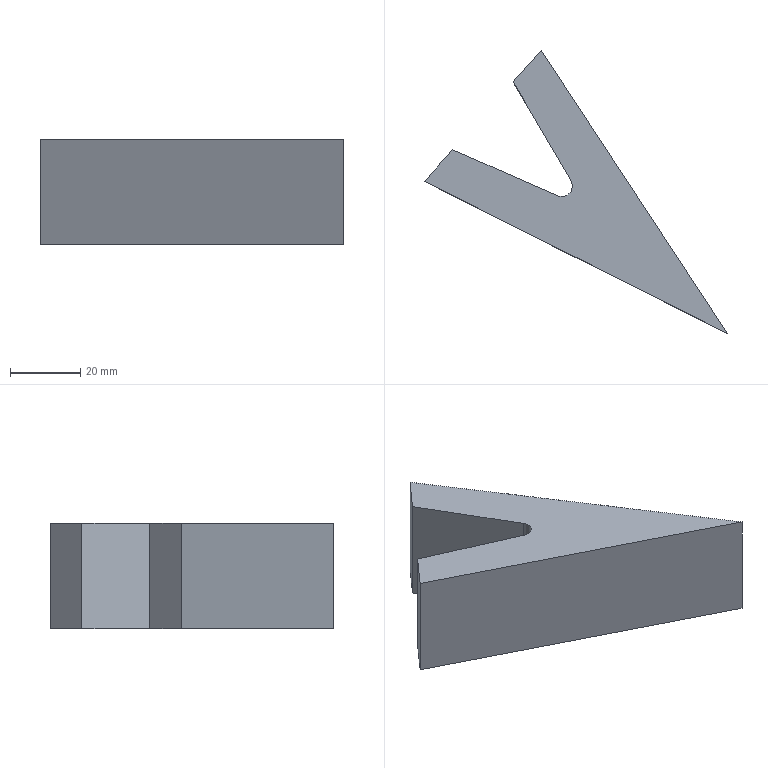Part | SolidWorks | features SavedExtBody 1 | 1 solid | 9 faces | box 85.955 x 80.416 x 30 mm | volume 54551 mm3 | plane 8 | cylinder 1 | commonest cylinder face diameters 6 x1
STEP:
#1=CARTESIAN_POINT('',(612.794,-213.858,-165.));
#2=VERTEX_POINT('',#1);
#3=CARTESIAN_POINT('',(608.998,-218.118,-165.));
#4=VERTEX_POINT('',#3);
#5=CARTESIAN_POINT('',(610.204,-215.371,-165.));
#6=DIRECTION('',(0.,0.,-1.));
#7=DIRECTION('',(1.,0.,0.));
#8=AXIS2_PLACEMENT_3D('',#5,#6,#7);
#9=CIRCLE('',#8,3.);
#10=EDGE_CURVE('',#2,#4,#9,.T.);
#11=ORIENTED_EDGE('',*,*,#10,.T.);
#12=CARTESIAN_POINT('',(608.998,-218.118,-135.));
#13=VERTEX_POINT('',#12);
#14=CARTESIAN_POINT('',(608.998,-218.118,-135.));
#15=DIRECTION('',(0.,0.,-1.));
#16=VECTOR('',#15,1000.);
#17=LINE('',#14,#16);
#18=EDGE_CURVE('',#13,#4,#17,.T.);
#19=ORIENTED_EDGE('',*,*,#18,.F.);
#20=CARTESIAN_POINT('',(612.794,-213.858,-135.));
#21=VERTEX_POINT('',#20);
#22=CARTESIAN_POINT('',(610.204,-215.371,-135.));
#23=DIRECTION('',(0.,0.,-1.));
#24=DIRECTION('',(1.,0.,0.));
#25=AXIS2_PLACEMENT_3D('',#22,#23,#24);
#26=CIRCLE('',#25,3.);
#27=EDGE_CURVE('',#21,#13,#26,.T.);
#28=ORIENTED_EDGE('',*,*,#27,.F.);
#29=CARTESIAN_POINT('',(612.794,-213.858,-135.));
#30=DIRECTION('',(0.,0.,-1.));
#31=VECTOR('',#30,1000.);
#32=LINE('',#29,#31);
#33=EDGE_CURVE('',#21,#2,#32,.T.);
#34=ORIENTED_EDGE('',*,*,#33,.T.);
#35=EDGE_LOOP('',(#11,#19,#28,#34));
#36=FACE_OUTER_BOUND('',#35,.T.);
#37=CARTESIAN_POINT('',(610.204,-215.371,-135.));
#38=DIRECTION('',(0.,0.,-1.));
#39=DIRECTION('',(-1.,0.,0.));
#40=AXIS2_PLACEMENT_3D('',#37,#38,#39);
#41=CYLINDRICAL_SURFACE('',#40,3.);
#42=ADVANCED_FACE('',(#36),#41,.F.);
#43=CARTESIAN_POINT('',(579.222,-205.048,-165.));
#44=VERTEX_POINT('',#43);
#45=CARTESIAN_POINT('',(579.222,-205.048,-165.));
#46=DIRECTION('',(-0.9157,0.4019,0.));
#47=VECTOR('',#46,1000.);
#48=LINE('',#45,#47);
#49=EDGE_CURVE('',#4,#44,#48,.T.);
#50=ORIENTED_EDGE('',*,*,#49,.T.);
#51=CARTESIAN_POINT('',(579.222,-205.048,-135.));
#52=VERTEX_POINT('',#51);
#53=CARTESIAN_POINT('',(579.222,-205.048,-135.));
#54=DIRECTION('',(0.,0.,-1.));
#55=VECTOR('',#54,1000.);
#56=LINE('',#53,#55);
#57=EDGE_CURVE('',#52,#44,#56,.T.);
#58=ORIENTED_EDGE('',*,*,#57,.F.);
#59=CARTESIAN_POINT('',(579.222,-205.048,-135.));
#60=DIRECTION('',(-0.9157,0.4019,0.));
#61=VECTOR('',#60,1000.);
#62=LINE('',#59,#61);
#63=EDGE_CURVE('',#13,#52,#62,.T.);
#64=ORIENTED_EDGE('',*,*,#63,.F.);
#65=ORIENTED_EDGE('',*,*,#18,.T.);
#66=EDGE_LOOP('',(#50,#58,#64,#65));
#67=FACE_OUTER_BOUND('',#66,.T.);
#68=CARTESIAN_POINT('',(579.222,-205.048,-135.));
#69=DIRECTION('',(-0.4019,-0.9157,0.));
#70=DIRECTION('',(0.9157,-0.4019,0.));
#71=AXIS2_PLACEMENT_3D('',#68,#69,#70);
#72=PLANE('',#71);
#73=ADVANCED_FACE('',(#67),#72,.F.);
#74=CARTESIAN_POINT('',(571.239,-214.007,-165.));
#75=VERTEX_POINT('',#74);
#76=CARTESIAN_POINT('',(571.239,-214.007,-165.));
#77=DIRECTION('',(-0.6652,-0.7466,0.));
#78=VECTOR('',#77,1000.);
#79=LINE('',#76,#78);
#80=EDGE_CURVE('',#44,#75,#79,.T.);
#81=ORIENTED_EDGE('',*,*,#80,.T.);
#82=CARTESIAN_POINT('',(571.239,-214.007,-135.));
#83=VERTEX_POINT('',#82);
#84=CARTESIAN_POINT('',(571.239,-214.007,-135.));
#85=DIRECTION('',(0.,0.,-1.));
#86=VECTOR('',#85,1000.);
#87=LINE('',#84,#86);
#88=EDGE_CURVE('',#83,#75,#87,.T.);
#89=ORIENTED_EDGE('',*,*,#88,.F.);
#90=CARTESIAN_POINT('',(571.239,-214.007,-135.));
#91=DIRECTION('',(-0.6652,-0.7466,0.));
#92=VECTOR('',#91,1000.);
#93=LINE('',#90,#92);
#94=EDGE_CURVE('',#52,#83,#93,.T.);
#95=ORIENTED_EDGE('',*,*,#94,.F.);
#96=ORIENTED_EDGE('',*,*,#57,.T.);
#97=EDGE_LOOP('',(#81,#89,#95,#96));
#98=FACE_OUTER_BOUND('',#97,.T.);
#99=CARTESIAN_POINT('',(571.239,-214.007,-135.));
#100=DIRECTION('',(0.7466,-0.6652,0.));
#101=DIRECTION('',(0.6652,0.7466,0.));
#102=AXIS2_PLACEMENT_3D('',#99,#100,#101);
#103=PLANE('',#102);
#104=ADVANCED_FACE('',(#98),#103,.F.);
#105=CARTESIAN_POINT('',(657.194,-257.238,-165.));
#106=VERTEX_POINT('',#105);
#107=CARTESIAN_POINT('',(657.194,-257.238,-165.));
#108=DIRECTION('',(0.8934,-0.4493,0.));
#109=VECTOR('',#108,1000.);
#110=LINE('',#107,#109);
#111=EDGE_CURVE('',#75,#106,#110,.T.);
#112=ORIENTED_EDGE('',*,*,#111,.T.);
#113=CARTESIAN_POINT('',(657.194,-257.238,-135.));
#114=VERTEX_POINT('',#113);
#115=CARTESIAN_POINT('',(657.194,-257.238,-135.));
#116=DIRECTION('',(0.,0.,-1.));
#117=VECTOR('',#116,1000.);
#118=LINE('',#115,#117);
#119=EDGE_CURVE('',#114,#106,#118,.T.);
#120=ORIENTED_EDGE('',*,*,#119,.F.);
#121=CARTESIAN_POINT('',(657.194,-257.238,-135.));
#122=DIRECTION('',(0.8934,-0.4493,0.));
#123=VECTOR('',#122,1000.);
#124=LINE('',#121,#123);
#125=EDGE_CURVE('',#83,#114,#124,.T.);
#126=ORIENTED_EDGE('',*,*,#125,.F.);
#127=ORIENTED_EDGE('',*,*,#88,.T.);
#128=EDGE_LOOP('',(#112,#120,#126,#127));
#129=FACE_OUTER_BOUND('',#128,.T.);
#130=CARTESIAN_POINT('',(657.194,-257.238,-135.));
#131=DIRECTION('',(0.4493,0.8934,0.));
#132=DIRECTION('',(-0.8934,0.4493,0.));
#133=AXIS2_PLACEMENT_3D('',#130,#131,#132);
#134=PLANE('',#133);
#135=ADVANCED_FACE('',(#129),#134,.F.);
#136=CARTESIAN_POINT('',(604.37,-176.822,-165.));
#137=VERTEX_POINT('',#136);
#138=CARTESIAN_POINT('',(604.37,-176.822,-165.));
#139=DIRECTION('',(-0.549,0.8358,0.));
#140=VECTOR('',#139,1000.);
#141=LINE('',#138,#140);
#142=EDGE_CURVE('',#106,#137,#141,.T.);
#143=ORIENTED_EDGE('',*,*,#142,.T.);
#144=CARTESIAN_POINT('',(604.37,-176.822,-135.));
#145=VERTEX_POINT('',#144);
#146=CARTESIAN_POINT('',(604.37,-176.822,-135.));
#147=DIRECTION('',(0.,0.,-1.));
#148=VECTOR('',#147,1000.);
#149=LINE('',#146,#148);
#150=EDGE_CURVE('',#145,#137,#149,.T.);
#151=ORIENTED_EDGE('',*,*,#150,.F.);
#152=CARTESIAN_POINT('',(604.37,-176.822,-135.));
#153=DIRECTION('',(-0.549,0.8358,0.));
#154=VECTOR('',#153,1000.);
#155=LINE('',#152,#154);
#156=EDGE_CURVE('',#114,#145,#155,.T.);
#157=ORIENTED_EDGE('',*,*,#156,.F.);
#158=ORIENTED_EDGE('',*,*,#119,.T.);
#159=EDGE_LOOP('',(#143,#151,#157,#158));
#160=FACE_OUTER_BOUND('',#159,.T.);
#161=CARTESIAN_POINT('',(604.37,-176.822,-135.));
#162=DIRECTION('',(-0.8358,-0.549,0.));
#163=DIRECTION('',(0.549,-0.8358,0.));
#164=AXIS2_PLACEMENT_3D('',#161,#162,#163);
#165=PLANE('',#164);
#166=ADVANCED_FACE('',(#160),#165,.F.);
#167=CARTESIAN_POINT('',(596.387,-185.781,-165.));
#168=VERTEX_POINT('',#167);
#169=CARTESIAN_POINT('',(596.387,-185.781,-165.));
#170=DIRECTION('',(-0.6652,-0.7466,0.));
#171=VECTOR('',#170,1000.);
#172=LINE('',#169,#171);
#173=EDGE_CURVE('',#137,#168,#172,.T.);
#174=ORIENTED_EDGE('',*,*,#173,.T.);
#175=CARTESIAN_POINT('',(596.387,-185.781,-135.));
#176=VERTEX_POINT('',#175);
#177=CARTESIAN_POINT('',(596.387,-185.781,-135.));
#178=DIRECTION('',(0.,0.,-1.));
#179=VECTOR('',#178,1000.);
#180=LINE('',#177,#179);
#181=EDGE_CURVE('',#176,#168,#180,.T.);
#182=ORIENTED_EDGE('',*,*,#181,.F.);
#183=CARTESIAN_POINT('',(596.387,-185.781,-135.));
#184=DIRECTION('',(-0.6652,-0.7466,0.));
#185=VECTOR('',#184,1000.);
#186=LINE('',#183,#185);
#187=EDGE_CURVE('',#145,#176,#186,.T.);
#188=ORIENTED_EDGE('',*,*,#187,.F.);
#189=ORIENTED_EDGE('',*,*,#150,.T.);
#190=EDGE_LOOP('',(#174,#182,#188,#189));
#191=FACE_OUTER_BOUND('',#190,.T.);
#192=CARTESIAN_POINT('',(596.387,-185.781,-135.));
#193=DIRECTION('',(0.7466,-0.6652,0.));
#194=DIRECTION('',(0.6652,0.7466,0.));
#195=AXIS2_PLACEMENT_3D('',#192,#193,#194);
#196=PLANE('',#195);
#197=ADVANCED_FACE('',(#191),#196,.F.);
#198=CARTESIAN_POINT('',(612.794,-213.858,-165.));
#199=DIRECTION('',(0.5045,-0.8634,0.));
#200=VECTOR('',#199,1000.);
#201=LINE('',#198,#200);
#202=EDGE_CURVE('',#168,#2,#201,.T.);
#203=ORIENTED_EDGE('',*,*,#202,.T.);
#204=ORIENTED_EDGE('',*,*,#33,.F.);
#205=CARTESIAN_POINT('',(612.794,-213.858,-135.));
#206=DIRECTION('',(0.5045,-0.8634,0.));
#207=VECTOR('',#206,1000.);
#208=LINE('',#205,#207);
#209=EDGE_CURVE('',#176,#21,#208,.T.);
#210=ORIENTED_EDGE('',*,*,#209,.F.);
#211=ORIENTED_EDGE('',*,*,#181,.T.);
#212=EDGE_LOOP('',(#203,#204,#210,#211));
#213=FACE_OUTER_BOUND('',#212,.T.);
#214=CARTESIAN_POINT('',(612.794,-213.858,-135.));
#215=DIRECTION('',(0.8634,0.5045,0.));
#216=DIRECTION('',(-0.5045,0.8634,0.));
#217=AXIS2_PLACEMENT_3D('',#214,#215,#216);
#218=PLANE('',#217);
#219=ADVANCED_FACE('',(#213),#218,.F.);
#220=ORIENTED_EDGE('',*,*,#27,.T.);
#221=ORIENTED_EDGE('',*,*,#63,.T.);
#222=ORIENTED_EDGE('',*,*,#94,.T.);
#223=ORIENTED_EDGE('',*,*,#125,.T.);
#224=ORIENTED_EDGE('',*,*,#156,.T.);
#225=ORIENTED_EDGE('',*,*,#187,.T.);
#226=ORIENTED_EDGE('',*,*,#209,.T.);
#227=EDGE_LOOP('',(#220,#221,#222,#223,#224,#225,#226));
#228=FACE_OUTER_BOUND('',#227,.T.);
#229=CARTESIAN_POINT('',(610.204,-215.371,-135.));
#230=DIRECTION('',(0.,0.,1.));
#231=DIRECTION('',(1.,0.,0.));
#232=AXIS2_PLACEMENT_3D('',#229,#230,#231);
#233=PLANE('',#232);
#234=ADVANCED_FACE('',(#228),#233,.T.);
#235=ORIENTED_EDGE('',*,*,#10,.F.);
#236=ORIENTED_EDGE('',*,*,#202,.F.);
#237=ORIENTED_EDGE('',*,*,#173,.F.);
#238=ORIENTED_EDGE('',*,*,#142,.F.);
#239=ORIENTED_EDGE('',*,*,#111,.F.);
#240=ORIENTED_EDGE('',*,*,#80,.F.);
#241=ORIENTED_EDGE('',*,*,#49,.F.);
#242=EDGE_LOOP('',(#235,#236,#237,#238,#239,#240,#241));
#243=FACE_OUTER_BOUND('',#242,.T.);
#244=CARTESIAN_POINT('',(610.204,-215.371,-165.));
#245=DIRECTION('',(0.,0.,1.));
#246=DIRECTION('',(1.,0.,0.));
#247=AXIS2_PLACEMENT_3D('',#244,#245,#246);
#248=PLANE('',#247);
#249=ADVANCED_FACE('',(#243),#248,.F.);
#250=CLOSED_SHELL('',(#42,#73,#104,#135,#166,#197,#219,#234,#249));
#251=MANIFOLD_SOLID_BREP('',#250);
#252=CARTESIAN_POINT('',(0.,0.,0.));
#253=DIRECTION('',(0.,0.,1.));
#254=DIRECTION('',(1.,0.,0.));
#255=AXIS2_PLACEMENT_3D('',#252,#253,#254);
#256=(LENGTH_UNIT()NAMED_UNIT(*)SI_UNIT(.MILLI.,.METRE.));
#257=UNCERTAINTY_MEASURE_WITH_UNIT(LENGTH_MEASURE(0.00001),#256,'','');
#258=(NAMED_UNIT(*)PLANE_ANGLE_UNIT()SI_UNIT($,.RADIAN.));
#259=(NAMED_UNIT(*)SI_UNIT($,.STERADIAN.)SOLID_ANGLE_UNIT());
#260=(GEOMETRIC_REPRESENTATION_CONTEXT(3)GLOBAL_UNCERTAINTY_ASSIGNED_CONTEXT((#257))GLOBAL_UNIT_ASSIGNED_CONTEXT((#256,#258,#259))REPRESENTATION_CONTEXT('',''));
#261=ADVANCED_BREP_SHAPE_REPRESENTATION('',(#251,#255),#260);